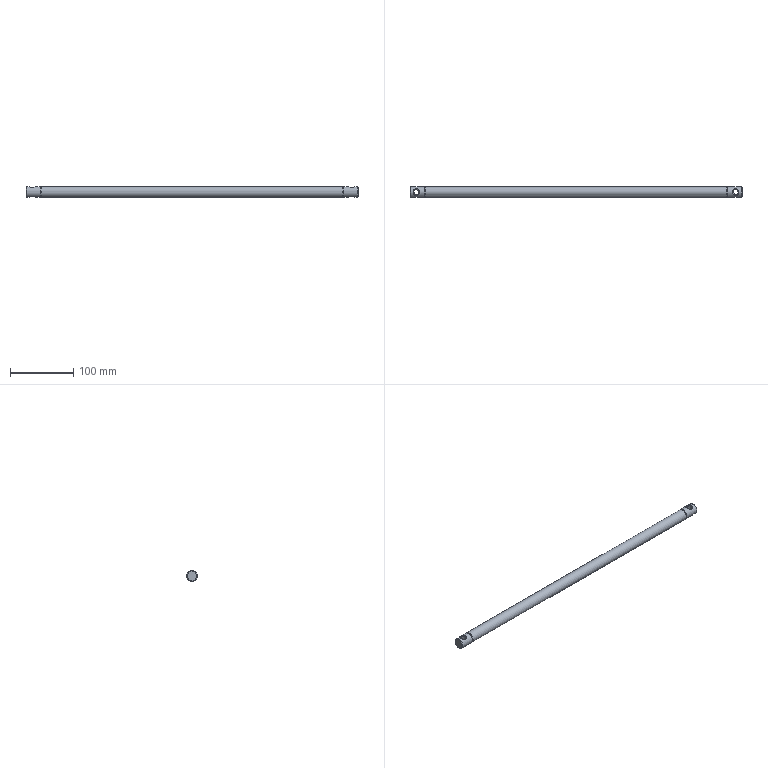Part | STEP file | 610B0802 | 1 solid | 19 faces | box 523 x 17 x 17 mm | volume 116777 mm3 | cylinder 7 | plane 6 | spline 4 | cone 2 | commonest cylinder face diameters 17 x3 8 x2 16 x2